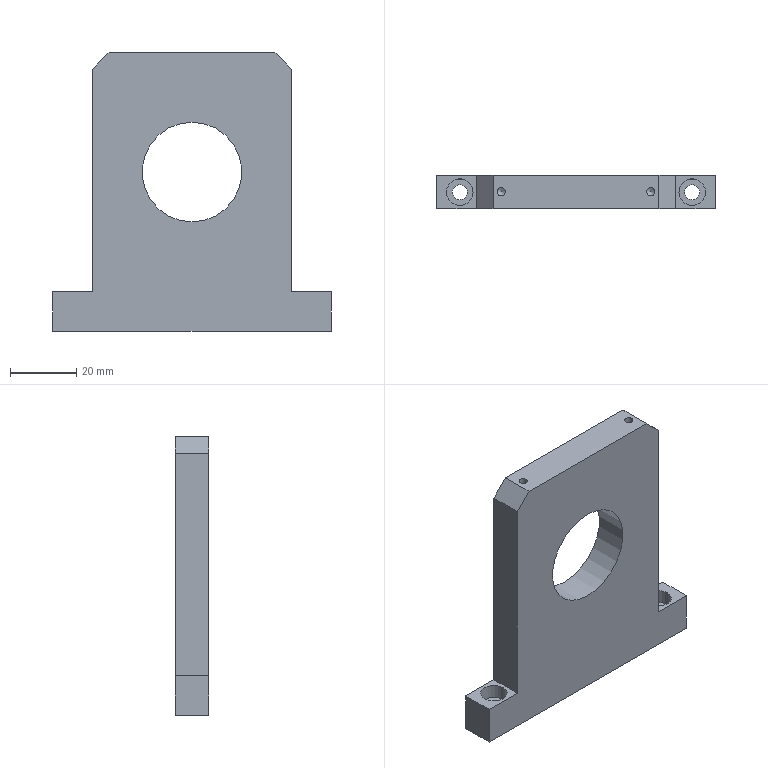Part | NX | 1 solid | 23 faces | box 84 x 10 x 84 mm | volume 45201 mm3 | plane 14 | cylinder 7 | cone 2 | commonest cylinder face diameters 2.5 x2 4.5 x2 8 x2 30 x1
STEP:
#1=CARTESIAN_POINT('',(30.,10.,31.));
#2=VERTEX_POINT('',#1);
#3=CARTESIAN_POINT('',(30.,10.,-36.));
#4=VERTEX_POINT('',#3);
#5=CARTESIAN_POINT('',(30.,10.,36.));
#6=DIRECTION('',(0.,0.,-1.));
#7=VECTOR('',#6,1000.);
#8=LINE('',#5,#7);
#9=EDGE_CURVE('',#2,#4,#8,.T.);
#10=ORIENTED_EDGE('',*,*,#9,.F.);
#11=CARTESIAN_POINT('',(30.,0.,31.));
#12=VERTEX_POINT('',#11);
#13=CARTESIAN_POINT('',(30.,10.,31.));
#14=DIRECTION('',(0.,-1.,0.));
#15=VECTOR('',#14,1000.);
#16=LINE('',#13,#15);
#17=EDGE_CURVE('',#2,#12,#16,.T.);
#18=ORIENTED_EDGE('',*,*,#17,.T.);
#19=CARTESIAN_POINT('',(30.,0.,-36.));
#20=VERTEX_POINT('',#19);
#21=CARTESIAN_POINT('',(30.,0.,36.));
#22=DIRECTION('',(0.,0.,-1.));
#23=VECTOR('',#22,1000.);
#24=LINE('',#21,#23);
#25=EDGE_CURVE('',#12,#20,#24,.T.);
#26=ORIENTED_EDGE('',*,*,#25,.T.);
#27=CARTESIAN_POINT('',(30.,10.,-36.));
#28=DIRECTION('',(0.,-1.,0.));
#29=VECTOR('',#28,1000.);
#30=LINE('',#27,#29);
#31=EDGE_CURVE('',#4,#20,#30,.T.);
#32=ORIENTED_EDGE('',*,*,#31,.F.);
#33=EDGE_LOOP('',(#10,#18,#26,#32));
#34=FACE_BOUND('',#33,.T.);
#35=CARTESIAN_POINT('',(30.,10.,36.));
#36=DIRECTION('',(-1.,0.,0.));
#37=DIRECTION('',(0.,0.,1.));
#38=AXIS2_PLACEMENT_3D('',#35,#36,#37);
#39=PLANE('',#38);
#40=ADVANCED_FACE('',(#34),#39,.F.);
#41=CARTESIAN_POINT('',(-30.,0.,-36.));
#42=VERTEX_POINT('',#41);
#43=CARTESIAN_POINT('',(-30.,0.,31.));
#44=VERTEX_POINT('',#43);
#45=CARTESIAN_POINT('',(-30.,0.,36.));
#46=DIRECTION('',(0.,0.,1.));
#47=VECTOR('',#46,1000.);
#48=LINE('',#45,#47);
#49=EDGE_CURVE('',#42,#44,#48,.T.);
#50=ORIENTED_EDGE('',*,*,#49,.T.);
#51=CARTESIAN_POINT('',(-30.,10.,31.));
#52=VERTEX_POINT('',#51);
#53=CARTESIAN_POINT('',(-30.,10.,31.));
#54=DIRECTION('',(0.,1.,0.));
#55=VECTOR('',#54,1000.);
#56=LINE('',#53,#55);
#57=EDGE_CURVE('',#44,#52,#56,.T.);
#58=ORIENTED_EDGE('',*,*,#57,.T.);
#59=CARTESIAN_POINT('',(-30.,10.,-36.));
#60=VERTEX_POINT('',#59);
#61=CARTESIAN_POINT('',(-30.,10.,36.));
#62=DIRECTION('',(0.,0.,1.));
#63=VECTOR('',#62,1000.);
#64=LINE('',#61,#63);
#65=EDGE_CURVE('',#60,#52,#64,.T.);
#66=ORIENTED_EDGE('',*,*,#65,.F.);
#67=CARTESIAN_POINT('',(-30.,10.,-36.));
#68=DIRECTION('',(0.,-1.,0.));
#69=VECTOR('',#68,1000.);
#70=LINE('',#67,#69);
#71=EDGE_CURVE('',#60,#42,#70,.T.);
#72=ORIENTED_EDGE('',*,*,#71,.T.);
#73=EDGE_LOOP('',(#50,#58,#66,#72));
#74=FACE_BOUND('',#73,.T.);
#75=CARTESIAN_POINT('',(-30.,10.,36.));
#76=DIRECTION('',(1.,0.,0.));
#77=DIRECTION('',(0.,0.,-1.));
#78=AXIS2_PLACEMENT_3D('',#75,#76,#77);
#79=PLANE('',#78);
#80=ADVANCED_FACE('',(#74),#79,.F.);
#81=CARTESIAN_POINT('',(-21.25,5.,36.));
#82=VERTEX_POINT('',#81);
#83=CARTESIAN_POINT('',(-22.5,5.,36.));
#84=DIRECTION('',(0.,0.,1.));
#85=DIRECTION('',(1.,0.,0.));
#86=AXIS2_PLACEMENT_3D('',#83,#84,#85);
#87=CIRCLE('',#86,1.25);
#88=EDGE_CURVE('',#82,#82,#87,.T.);
#89=ORIENTED_EDGE('',*,*,#88,.F.);
#90=EDGE_LOOP('',(#89));
#91=FACE_BOUND('',#90,.T.);
#92=CARTESIAN_POINT('',(23.75,5.,36.));
#93=VERTEX_POINT('',#92);
#94=CARTESIAN_POINT('',(22.5,5.,36.));
#95=DIRECTION('',(0.,0.,1.));
#96=DIRECTION('',(1.,0.,0.));
#97=AXIS2_PLACEMENT_3D('',#94,#95,#96);
#98=CIRCLE('',#97,1.25);
#99=EDGE_CURVE('',#93,#93,#98,.T.);
#100=ORIENTED_EDGE('',*,*,#99,.F.);
#101=EDGE_LOOP('',(#100));
#102=FACE_BOUND('',#101,.T.);
#103=CARTESIAN_POINT('',(-25.,0.,36.));
#104=VERTEX_POINT('',#103);
#105=CARTESIAN_POINT('',(25.,0.,36.));
#106=VERTEX_POINT('',#105);
#107=CARTESIAN_POINT('',(-30.,0.,36.));
#108=DIRECTION('',(1.,0.,0.));
#109=VECTOR('',#108,1000.);
#110=LINE('',#107,#109);
#111=EDGE_CURVE('',#104,#106,#110,.T.);
#112=ORIENTED_EDGE('',*,*,#111,.T.);
#113=CARTESIAN_POINT('',(25.,10.,36.));
#114=VERTEX_POINT('',#113);
#115=CARTESIAN_POINT('',(25.,10.,36.));
#116=DIRECTION('',(0.,1.,0.));
#117=VECTOR('',#116,1000.);
#118=LINE('',#115,#117);
#119=EDGE_CURVE('',#106,#114,#118,.T.);
#120=ORIENTED_EDGE('',*,*,#119,.T.);
#121=CARTESIAN_POINT('',(-25.,10.,36.));
#122=VERTEX_POINT('',#121);
#123=CARTESIAN_POINT('',(-30.,10.,36.));
#124=DIRECTION('',(1.,0.,0.));
#125=VECTOR('',#124,1000.);
#126=LINE('',#123,#125);
#127=EDGE_CURVE('',#122,#114,#126,.T.);
#128=ORIENTED_EDGE('',*,*,#127,.F.);
#129=CARTESIAN_POINT('',(-25.,10.,36.));
#130=DIRECTION('',(0.,-1.,0.));
#131=VECTOR('',#130,1000.);
#132=LINE('',#129,#131);
#133=EDGE_CURVE('',#122,#104,#132,.T.);
#134=ORIENTED_EDGE('',*,*,#133,.T.);
#135=EDGE_LOOP('',(#112,#120,#128,#134));
#136=FACE_BOUND('',#135,.T.);
#137=CARTESIAN_POINT('',(-30.,10.,36.));
#138=DIRECTION('',(0.,0.,-1.));
#139=DIRECTION('',(-1.,0.,0.));
#140=AXIS2_PLACEMENT_3D('',#137,#138,#139);
#141=PLANE('',#140);
#142=ADVANCED_FACE('',(#91,#102,#136),#141,.F.);
#143=CARTESIAN_POINT('',(0.,10.,-15.));
#144=VERTEX_POINT('',#143);
#145=CARTESIAN_POINT('',(0.,10.,0.));
#146=DIRECTION('',(0.,-1.,0.));
#147=DIRECTION('',(0.,0.,-1.));
#148=AXIS2_PLACEMENT_3D('',#145,#146,#147);
#149=CIRCLE('',#148,15.);
#150=EDGE_CURVE('',#144,#144,#149,.T.);
#151=ORIENTED_EDGE('',*,*,#150,.T.);
#152=EDGE_LOOP('',(#151));
#153=FACE_BOUND('',#152,.T.);
#154=ORIENTED_EDGE('',*,*,#127,.T.);
#155=CARTESIAN_POINT('',(30.,10.,31.));
#156=DIRECTION('',(-0.7071,0.,0.7071));
#157=VECTOR('',#156,1000.);
#158=LINE('',#155,#157);
#159=EDGE_CURVE('',#114,#2,#158,.F.);
#160=ORIENTED_EDGE('',*,*,#159,.T.);
#161=ORIENTED_EDGE('',*,*,#9,.T.);
#162=CARTESIAN_POINT('',(42.,10.,-36.));
#163=VERTEX_POINT('',#162);
#164=CARTESIAN_POINT('',(-42.,10.,-36.));
#165=DIRECTION('',(1.,0.,0.));
#166=VECTOR('',#165,1000.);
#167=LINE('',#164,#166);
#168=EDGE_CURVE('',#4,#163,#167,.T.);
#169=ORIENTED_EDGE('',*,*,#168,.T.);
#170=CARTESIAN_POINT('',(42.,10.,-48.));
#171=VERTEX_POINT('',#170);
#172=CARTESIAN_POINT('',(42.,10.,-48.));
#173=DIRECTION('',(0.,0.,-1.));
#174=VECTOR('',#173,1000.);
#175=LINE('',#172,#174);
#176=EDGE_CURVE('',#163,#171,#175,.T.);
#177=ORIENTED_EDGE('',*,*,#176,.T.);
#178=CARTESIAN_POINT('',(-42.,10.,-48.));
#179=VERTEX_POINT('',#178);
#180=CARTESIAN_POINT('',(-42.,10.,-48.));
#181=DIRECTION('',(-1.,0.,0.));
#182=VECTOR('',#181,1000.);
#183=LINE('',#180,#182);
#184=EDGE_CURVE('',#171,#179,#183,.T.);
#185=ORIENTED_EDGE('',*,*,#184,.T.);
#186=CARTESIAN_POINT('',(-42.,10.,-36.));
#187=VERTEX_POINT('',#186);
#188=CARTESIAN_POINT('',(-42.,10.,-48.));
#189=DIRECTION('',(0.,0.,1.));
#190=VECTOR('',#189,1000.);
#191=LINE('',#188,#190);
#192=EDGE_CURVE('',#179,#187,#191,.T.);
#193=ORIENTED_EDGE('',*,*,#192,.T.);
#194=CARTESIAN_POINT('',(-42.,10.,-36.));
#195=DIRECTION('',(1.,0.,0.));
#196=VECTOR('',#195,1000.);
#197=LINE('',#194,#196);
#198=EDGE_CURVE('',#187,#60,#197,.T.);
#199=ORIENTED_EDGE('',*,*,#198,.T.);
#200=ORIENTED_EDGE('',*,*,#65,.T.);
#201=CARTESIAN_POINT('',(-25.,10.,36.));
#202=DIRECTION('',(-0.7071,0.,-0.7071));
#203=VECTOR('',#202,1000.);
#204=LINE('',#201,#203);
#205=EDGE_CURVE('',#52,#122,#204,.F.);
#206=ORIENTED_EDGE('',*,*,#205,.T.);
#207=EDGE_LOOP('',(#154,#160,#161,#169,#177,#185,#193,#199,#200,#206));
#208=FACE_BOUND('',#207,.T.);
#209=CARTESIAN_POINT('',(0.,10.,0.));
#210=DIRECTION('',(0.,-1.,0.));
#211=DIRECTION('',(0.,0.,-1.));
#212=AXIS2_PLACEMENT_3D('',#209,#210,#211);
#213=PLANE('',#212);
#214=ADVANCED_FACE('',(#153,#208),#213,.F.);
#215=CARTESIAN_POINT('',(0.,0.,-15.));
#216=VERTEX_POINT('',#215);
#217=CARTESIAN_POINT('',(0.,0.,0.));
#218=DIRECTION('',(0.,-1.,0.));
#219=DIRECTION('',(0.,0.,-1.));
#220=AXIS2_PLACEMENT_3D('',#217,#218,#219);
#221=CIRCLE('',#220,15.);
#222=EDGE_CURVE('',#216,#216,#221,.T.);
#223=ORIENTED_EDGE('',*,*,#222,.F.);
#224=EDGE_LOOP('',(#223));
#225=FACE_BOUND('',#224,.T.);
#226=ORIENTED_EDGE('',*,*,#25,.F.);
#227=CARTESIAN_POINT('',(30.5,0.,30.5));
#228=DIRECTION('',(0.7071,0.,-0.7071));
#229=VECTOR('',#228,1000.);
#230=LINE('',#227,#229);
#231=EDGE_CURVE('',#12,#106,#230,.F.);
#232=ORIENTED_EDGE('',*,*,#231,.T.);
#233=ORIENTED_EDGE('',*,*,#111,.F.);
#234=CARTESIAN_POINT('',(-30.5,0.,30.5));
#235=DIRECTION('',(0.7071,0.,0.7071));
#236=VECTOR('',#235,1000.);
#237=LINE('',#234,#236);
#238=EDGE_CURVE('',#104,#44,#237,.F.);
#239=ORIENTED_EDGE('',*,*,#238,.T.);
#240=ORIENTED_EDGE('',*,*,#49,.F.);
#241=CARTESIAN_POINT('',(-42.,0.,-36.));
#242=VERTEX_POINT('',#241);
#243=CARTESIAN_POINT('',(-42.,0.,-36.));
#244=DIRECTION('',(1.,0.,0.));
#245=VECTOR('',#244,1000.);
#246=LINE('',#243,#245);
#247=EDGE_CURVE('',#242,#42,#246,.T.);
#248=ORIENTED_EDGE('',*,*,#247,.F.);
#249=CARTESIAN_POINT('',(-42.,0.,-48.));
#250=VERTEX_POINT('',#249);
#251=CARTESIAN_POINT('',(-42.,0.,-48.));
#252=DIRECTION('',(0.,0.,1.));
#253=VECTOR('',#252,1000.);
#254=LINE('',#251,#253);
#255=EDGE_CURVE('',#250,#242,#254,.T.);
#256=ORIENTED_EDGE('',*,*,#255,.F.);
#257=CARTESIAN_POINT('',(42.,0.,-48.));
#258=VERTEX_POINT('',#257);
#259=CARTESIAN_POINT('',(-42.,0.,-48.));
#260=DIRECTION('',(-1.,0.,0.));
#261=VECTOR('',#260,1000.);
#262=LINE('',#259,#261);
#263=EDGE_CURVE('',#258,#250,#262,.T.);
#264=ORIENTED_EDGE('',*,*,#263,.F.);
#265=CARTESIAN_POINT('',(42.,0.,-36.));
#266=VERTEX_POINT('',#265);
#267=CARTESIAN_POINT('',(42.,0.,-48.));
#268=DIRECTION('',(0.,0.,-1.));
#269=VECTOR('',#268,1000.);
#270=LINE('',#267,#269);
#271=EDGE_CURVE('',#266,#258,#270,.T.);
#272=ORIENTED_EDGE('',*,*,#271,.F.);
#273=CARTESIAN_POINT('',(-42.,0.,-36.));
#274=DIRECTION('',(1.,0.,0.));
#275=VECTOR('',#274,1000.);
#276=LINE('',#273,#275);
#277=EDGE_CURVE('',#20,#266,#276,.T.);
#278=ORIENTED_EDGE('',*,*,#277,.F.);
#279=EDGE_LOOP('',(#226,#232,#233,#239,#240,#248,#256,#264,#272,#278));
#280=FACE_BOUND('',#279,.T.);
#281=CARTESIAN_POINT('',(0.,0.,0.));
#282=DIRECTION('',(0.,-1.,0.));
#283=DIRECTION('',(0.,0.,-1.));
#284=AXIS2_PLACEMENT_3D('',#281,#282,#283);
#285=PLANE('',#284);
#286=ADVANCED_FACE('',(#225,#280),#285,.T.);
#287=CARTESIAN_POINT('',(22.5,5.,27.749));
#288=VERTEX_POINT('',#287);
#289=VERTEX_LOOP('',#288);
#290=FACE_BOUND('',#289,.T.);
#291=CARTESIAN_POINT('',(23.75,5.,28.5));
#292=VERTEX_POINT('',#291);
#293=CARTESIAN_POINT('',(22.5,5.,28.5));
#294=DIRECTION('',(0.,0.,1.));
#295=DIRECTION('',(1.,0.,0.));
#296=AXIS2_PLACEMENT_3D('',#293,#294,#295);
#297=CIRCLE('',#296,1.25);
#298=EDGE_CURVE('',#292,#292,#297,.T.);
#299=ORIENTED_EDGE('',*,*,#298,.T.);
#300=EDGE_LOOP('',(#299));
#301=FACE_BOUND('',#300,.T.);
#302=CARTESIAN_POINT('',(22.5,5.,28.5));
#303=DIRECTION('',(0.,0.,1.));
#304=DIRECTION('',(1.,0.,0.));
#305=AXIS2_PLACEMENT_3D('',#302,#303,#304);
#306=CONICAL_SURFACE('',#305,1.25,1.03);
#307=ADVANCED_FACE('',(#290,#301),#306,.F.);
#308=ORIENTED_EDGE('',*,*,#298,.F.);
#309=EDGE_LOOP('',(#308));
#310=FACE_BOUND('',#309,.T.);
#311=ORIENTED_EDGE('',*,*,#99,.T.);
#312=EDGE_LOOP('',(#311));
#313=FACE_BOUND('',#312,.T.);
#314=CARTESIAN_POINT('',(22.5,5.,36.));
#315=DIRECTION('',(0.,0.,1.));
#316=DIRECTION('',(1.,0.,0.));
#317=AXIS2_PLACEMENT_3D('',#314,#315,#316);
#318=CYLINDRICAL_SURFACE('',#317,1.25);
#319=ADVANCED_FACE('',(#310,#313),#318,.F.);
#320=CARTESIAN_POINT('',(-22.5,5.,27.749));
#321=VERTEX_POINT('',#320);
#322=VERTEX_LOOP('',#321);
#323=FACE_BOUND('',#322,.T.);
#324=CARTESIAN_POINT('',(-21.25,5.,28.5));
#325=VERTEX_POINT('',#324);
#326=CARTESIAN_POINT('',(-22.5,5.,28.5));
#327=DIRECTION('',(0.,0.,1.));
#328=DIRECTION('',(1.,0.,0.));
#329=AXIS2_PLACEMENT_3D('',#326,#327,#328);
#330=CIRCLE('',#329,1.25);
#331=EDGE_CURVE('',#325,#325,#330,.T.);
#332=ORIENTED_EDGE('',*,*,#331,.T.);
#333=EDGE_LOOP('',(#332));
#334=FACE_BOUND('',#333,.T.);
#335=CARTESIAN_POINT('',(-22.5,5.,28.5));
#336=DIRECTION('',(0.,0.,1.));
#337=DIRECTION('',(1.,0.,0.));
#338=AXIS2_PLACEMENT_3D('',#335,#336,#337);
#339=CONICAL_SURFACE('',#338,1.25,1.03);
#340=ADVANCED_FACE('',(#323,#334),#339,.F.);
#341=ORIENTED_EDGE('',*,*,#331,.F.);
#342=EDGE_LOOP('',(#341));
#343=FACE_BOUND('',#342,.T.);
#344=ORIENTED_EDGE('',*,*,#88,.T.);
#345=EDGE_LOOP('',(#344));
#346=FACE_BOUND('',#345,.T.);
#347=CARTESIAN_POINT('',(-22.5,5.,36.));
#348=DIRECTION('',(0.,0.,1.));
#349=DIRECTION('',(1.,0.,0.));
#350=AXIS2_PLACEMENT_3D('',#347,#348,#349);
#351=CYLINDRICAL_SURFACE('',#350,1.25);
#352=ADVANCED_FACE('',(#343,#346),#351,.F.);
#353=ORIENTED_EDGE('',*,*,#150,.F.);
#354=EDGE_LOOP('',(#353));
#355=FACE_BOUND('',#354,.T.);
#356=ORIENTED_EDGE('',*,*,#222,.T.);
#357=EDGE_LOOP('',(#356));
#358=FACE_BOUND('',#357,.T.);
#359=CARTESIAN_POINT('',(0.,10.,0.));
#360=DIRECTION('',(0.,-1.,0.));
#361=DIRECTION('',(0.,0.,-1.));
#362=AXIS2_PLACEMENT_3D('',#359,#360,#361);
#363=CYLINDRICAL_SURFACE('',#362,15.);
#364=ADVANCED_FACE('',(#355,#358),#363,.F.);
#365=CARTESIAN_POINT('',(-31.,5.,-36.));
#366=VERTEX_POINT('',#365);
#367=CARTESIAN_POINT('',(-35.,5.,-36.));
#368=DIRECTION('',(0.,0.,1.));
#369=DIRECTION('',(1.,0.,0.));
#370=AXIS2_PLACEMENT_3D('',#367,#368,#369);
#371=CIRCLE('',#370,4.);
#372=EDGE_CURVE('',#366,#366,#371,.T.);
#373=ORIENTED_EDGE('',*,*,#372,.F.);
#374=EDGE_LOOP('',(#373));
#375=FACE_BOUND('',#374,.T.);
#376=ORIENTED_EDGE('',*,*,#71,.F.);
#377=ORIENTED_EDGE('',*,*,#198,.F.);
#378=CARTESIAN_POINT('',(-42.,-84.853,-36.));
#379=DIRECTION('',(0.,1.,0.));
#380=VECTOR('',#379,1000.);
#381=LINE('',#378,#380);
#382=EDGE_CURVE('',#242,#187,#381,.T.);
#383=ORIENTED_EDGE('',*,*,#382,.F.);
#384=ORIENTED_EDGE('',*,*,#247,.T.);
#385=EDGE_LOOP('',(#376,#377,#383,#384));
#386=FACE_BOUND('',#385,.T.);
#387=CARTESIAN_POINT('',(-42.,-84.853,-36.));
#388=DIRECTION('',(0.,0.,1.));
#389=DIRECTION('',(1.,0.,0.));
#390=AXIS2_PLACEMENT_3D('',#387,#388,#389);
#391=PLANE('',#390);
#392=ADVANCED_FACE('',(#375,#386),#391,.T.);
#393=CARTESIAN_POINT('',(-32.75,5.,-48.));
#394=VERTEX_POINT('',#393);
#395=CARTESIAN_POINT('',(-35.,5.,-48.));
#396=DIRECTION('',(0.,0.,1.));
#397=DIRECTION('',(1.,0.,0.));
#398=AXIS2_PLACEMENT_3D('',#395,#396,#397);
#399=CIRCLE('',#398,2.25);
#400=EDGE_CURVE('',#394,#394,#399,.T.);
#401=ORIENTED_EDGE('',*,*,#400,.T.);
#402=EDGE_LOOP('',(#401));
#403=FACE_BOUND('',#402,.T.);
#404=CARTESIAN_POINT('',(37.25,5.,-48.));
#405=VERTEX_POINT('',#404);
#406=CARTESIAN_POINT('',(35.,5.,-48.));
#407=DIRECTION('',(0.,0.,1.));
#408=DIRECTION('',(1.,0.,0.));
#409=AXIS2_PLACEMENT_3D('',#406,#407,#408);
#410=CIRCLE('',#409,2.25);
#411=EDGE_CURVE('',#405,#405,#410,.T.);
#412=ORIENTED_EDGE('',*,*,#411,.T.);
#413=EDGE_LOOP('',(#412));
#414=FACE_BOUND('',#413,.T.);
#415=CARTESIAN_POINT('',(42.,-84.853,-48.));
#416=DIRECTION('',(0.,1.,0.));
#417=VECTOR('',#416,1000.);
#418=LINE('',#415,#417);
#419=EDGE_CURVE('',#258,#171,#418,.T.);
#420=ORIENTED_EDGE('',*,*,#419,.F.);
#421=ORIENTED_EDGE('',*,*,#263,.T.);
#422=CARTESIAN_POINT('',(-42.,-84.853,-48.));
#423=DIRECTION('',(0.,1.,0.));
#424=VECTOR('',#423,1000.);
#425=LINE('',#422,#424);
#426=EDGE_CURVE('',#250,#179,#425,.T.);
#427=ORIENTED_EDGE('',*,*,#426,.T.);
#428=ORIENTED_EDGE('',*,*,#184,.F.);
#429=EDGE_LOOP('',(#420,#421,#427,#428));
#430=FACE_BOUND('',#429,.T.);
#431=CARTESIAN_POINT('',(-42.,-84.853,-48.));
#432=DIRECTION('',(0.,0.,-1.));
#433=DIRECTION('',(-1.,0.,0.));
#434=AXIS2_PLACEMENT_3D('',#431,#432,#433);
#435=PLANE('',#434);
#436=ADVANCED_FACE('',(#403,#414,#430),#435,.T.);
#437=ORIENTED_EDGE('',*,*,#426,.F.);
#438=ORIENTED_EDGE('',*,*,#255,.T.);
#439=ORIENTED_EDGE('',*,*,#382,.T.);
#440=ORIENTED_EDGE('',*,*,#192,.F.);
#441=EDGE_LOOP('',(#437,#438,#439,#440));
#442=FACE_BOUND('',#441,.T.);
#443=CARTESIAN_POINT('',(-42.,-84.853,-48.));
#444=DIRECTION('',(-1.,0.,0.));
#445=DIRECTION('',(0.,0.,1.));
#446=AXIS2_PLACEMENT_3D('',#443,#444,#445);
#447=PLANE('',#446);
#448=ADVANCED_FACE('',(#442),#447,.T.);
#449=CARTESIAN_POINT('',(39.,5.,-36.));
#450=VERTEX_POINT('',#449);
#451=CARTESIAN_POINT('',(35.,5.,-36.));
#452=DIRECTION('',(0.,0.,1.));
#453=DIRECTION('',(1.,0.,0.));
#454=AXIS2_PLACEMENT_3D('',#451,#452,#453);
#455=CIRCLE('',#454,4.);
#456=EDGE_CURVE('',#450,#450,#455,.T.);
#457=ORIENTED_EDGE('',*,*,#456,.F.);
#458=EDGE_LOOP('',(#457));
#459=FACE_BOUND('',#458,.T.);
#460=ORIENTED_EDGE('',*,*,#168,.F.);
#461=ORIENTED_EDGE('',*,*,#31,.T.);
#462=ORIENTED_EDGE('',*,*,#277,.T.);
#463=CARTESIAN_POINT('',(42.,-84.853,-36.));
#464=DIRECTION('',(0.,1.,0.));
#465=VECTOR('',#464,1000.);
#466=LINE('',#463,#465);
#467=EDGE_CURVE('',#266,#163,#466,.T.);
#468=ORIENTED_EDGE('',*,*,#467,.T.);
#469=EDGE_LOOP('',(#460,#461,#462,#468));
#470=FACE_BOUND('',#469,.T.);
#471=CARTESIAN_POINT('',(-42.,-84.853,-36.));
#472=DIRECTION('',(0.,0.,1.));
#473=DIRECTION('',(1.,0.,0.));
#474=AXIS2_PLACEMENT_3D('',#471,#472,#473);
#475=PLANE('',#474);
#476=ADVANCED_FACE('',(#459,#470),#475,.T.);
#477=ORIENTED_EDGE('',*,*,#467,.F.);
#478=ORIENTED_EDGE('',*,*,#271,.T.);
#479=ORIENTED_EDGE('',*,*,#419,.T.);
#480=ORIENTED_EDGE('',*,*,#176,.F.);
#481=EDGE_LOOP('',(#477,#478,#479,#480));
#482=FACE_BOUND('',#481,.T.);
#483=CARTESIAN_POINT('',(42.,-84.853,-48.));
#484=DIRECTION('',(1.,0.,0.));
#485=DIRECTION('',(0.,0.,-1.));
#486=AXIS2_PLACEMENT_3D('',#483,#484,#485);
#487=PLANE('',#486);
#488=ADVANCED_FACE('',(#482),#487,.T.);
#489=ORIENTED_EDGE('',*,*,#411,.F.);
#490=EDGE_LOOP('',(#489));
#491=FACE_BOUND('',#490,.T.);
#492=CARTESIAN_POINT('',(37.25,5.,-40.4));
#493=VERTEX_POINT('',#492);
#494=CARTESIAN_POINT('',(35.,5.,-40.4));
#495=DIRECTION('',(0.,0.,1.));
#496=DIRECTION('',(1.,0.,0.));
#497=AXIS2_PLACEMENT_3D('',#494,#495,#496);
#498=CIRCLE('',#497,2.25);
#499=EDGE_CURVE('',#493,#493,#498,.T.);
#500=ORIENTED_EDGE('',*,*,#499,.T.);
#501=EDGE_LOOP('',(#500));
#502=FACE_BOUND('',#501,.T.);
#503=CARTESIAN_POINT('',(35.,5.,-36.));
#504=DIRECTION('',(0.,0.,1.));
#505=DIRECTION('',(1.,0.,0.));
#506=AXIS2_PLACEMENT_3D('',#503,#504,#505);
#507=CYLINDRICAL_SURFACE('',#506,2.25);
#508=ADVANCED_FACE('',(#491,#502),#507,.F.);
#509=ORIENTED_EDGE('',*,*,#499,.F.);
#510=EDGE_LOOP('',(#509));
#511=FACE_BOUND('',#510,.T.);
#512=CARTESIAN_POINT('',(39.,5.,-40.4));
#513=VERTEX_POINT('',#512);
#514=CARTESIAN_POINT('',(35.,5.,-40.4));
#515=DIRECTION('',(0.,0.,1.));
#516=DIRECTION('',(1.,0.,0.));
#517=AXIS2_PLACEMENT_3D('',#514,#515,#516);
#518=CIRCLE('',#517,4.);
#519=EDGE_CURVE('',#513,#513,#518,.T.);
#520=ORIENTED_EDGE('',*,*,#519,.T.);
#521=EDGE_LOOP('',(#520));
#522=FACE_BOUND('',#521,.T.);
#523=CARTESIAN_POINT('',(37.25,5.,-40.4));
#524=DIRECTION('',(0.,0.,-1.));
#525=DIRECTION('',(-1.,0.,0.));
#526=AXIS2_PLACEMENT_3D('',#523,#524,#525);
#527=PLANE('',#526);
#528=ADVANCED_FACE('',(#511,#522),#527,.F.);
#529=ORIENTED_EDGE('',*,*,#519,.F.);
#530=EDGE_LOOP('',(#529));
#531=FACE_BOUND('',#530,.T.);
#532=ORIENTED_EDGE('',*,*,#456,.T.);
#533=EDGE_LOOP('',(#532));
#534=FACE_BOUND('',#533,.T.);
#535=CARTESIAN_POINT('',(35.,5.,-36.));
#536=DIRECTION('',(0.,0.,1.));
#537=DIRECTION('',(1.,0.,0.));
#538=AXIS2_PLACEMENT_3D('',#535,#536,#537);
#539=CYLINDRICAL_SURFACE('',#538,4.);
#540=ADVANCED_FACE('',(#531,#534),#539,.F.);
#541=ORIENTED_EDGE('',*,*,#400,.F.);
#542=EDGE_LOOP('',(#541));
#543=FACE_BOUND('',#542,.T.);
#544=CARTESIAN_POINT('',(-32.75,5.,-40.4));
#545=VERTEX_POINT('',#544);
#546=CARTESIAN_POINT('',(-35.,5.,-40.4));
#547=DIRECTION('',(0.,0.,1.));
#548=DIRECTION('',(1.,0.,0.));
#549=AXIS2_PLACEMENT_3D('',#546,#547,#548);
#550=CIRCLE('',#549,2.25);
#551=EDGE_CURVE('',#545,#545,#550,.T.);
#552=ORIENTED_EDGE('',*,*,#551,.T.);
#553=EDGE_LOOP('',(#552));
#554=FACE_BOUND('',#553,.T.);
#555=CARTESIAN_POINT('',(-35.,5.,-36.));
#556=DIRECTION('',(0.,0.,1.));
#557=DIRECTION('',(1.,0.,0.));
#558=AXIS2_PLACEMENT_3D('',#555,#556,#557);
#559=CYLINDRICAL_SURFACE('',#558,2.25);
#560=ADVANCED_FACE('',(#543,#554),#559,.F.);
#561=ORIENTED_EDGE('',*,*,#551,.F.);
#562=EDGE_LOOP('',(#561));
#563=FACE_BOUND('',#562,.T.);
#564=CARTESIAN_POINT('',(-31.,5.,-40.4));
#565=VERTEX_POINT('',#564);
#566=CARTESIAN_POINT('',(-35.,5.,-40.4));
#567=DIRECTION('',(0.,0.,1.));
#568=DIRECTION('',(1.,0.,0.));
#569=AXIS2_PLACEMENT_3D('',#566,#567,#568);
#570=CIRCLE('',#569,4.);
#571=EDGE_CURVE('',#565,#565,#570,.T.);
#572=ORIENTED_EDGE('',*,*,#571,.T.);
#573=EDGE_LOOP('',(#572));
#574=FACE_BOUND('',#573,.T.);
#575=CARTESIAN_POINT('',(-32.75,5.,-40.4));
#576=DIRECTION('',(0.,0.,-1.));
#577=DIRECTION('',(-1.,0.,0.));
#578=AXIS2_PLACEMENT_3D('',#575,#576,#577);
#579=PLANE('',#578);
#580=ADVANCED_FACE('',(#563,#574),#579,.F.);
#581=ORIENTED_EDGE('',*,*,#571,.F.);
#582=EDGE_LOOP('',(#581));
#583=FACE_BOUND('',#582,.T.);
#584=ORIENTED_EDGE('',*,*,#372,.T.);
#585=EDGE_LOOP('',(#584));
#586=FACE_BOUND('',#585,.T.);
#587=CARTESIAN_POINT('',(-35.,5.,-36.));
#588=DIRECTION('',(0.,0.,1.));
#589=DIRECTION('',(1.,0.,0.));
#590=AXIS2_PLACEMENT_3D('',#587,#588,#589);
#591=CYLINDRICAL_SURFACE('',#590,4.);
#592=ADVANCED_FACE('',(#583,#586),#591,.F.);
#593=ORIENTED_EDGE('',*,*,#159,.F.);
#594=ORIENTED_EDGE('',*,*,#119,.F.);
#595=ORIENTED_EDGE('',*,*,#231,.F.);
#596=ORIENTED_EDGE('',*,*,#17,.F.);
#597=EDGE_LOOP('',(#593,#594,#595,#596));
#598=FACE_BOUND('',#597,.T.);
#599=CARTESIAN_POINT('',(30.,10.,31.));
#600=DIRECTION('',(-0.7071,0.,-0.7071));
#601=DIRECTION('',(0.,-1.,0.));
#602=AXIS2_PLACEMENT_3D('',#599,#600,#601);
#603=PLANE('',#602);
#604=ADVANCED_FACE('',(#598),#603,.F.);
#605=ORIENTED_EDGE('',*,*,#205,.F.);
#606=ORIENTED_EDGE('',*,*,#57,.F.);
#607=ORIENTED_EDGE('',*,*,#238,.F.);
#608=ORIENTED_EDGE('',*,*,#133,.F.);
#609=EDGE_LOOP('',(#605,#606,#607,#608));
#610=FACE_BOUND('',#609,.T.);
#611=CARTESIAN_POINT('',(-25.,10.,36.));
#612=DIRECTION('',(0.7071,0.,-0.7071));
#613=DIRECTION('',(0.,-1.,0.));
#614=AXIS2_PLACEMENT_3D('',#611,#612,#613);
#615=PLANE('',#614);
#616=ADVANCED_FACE('',(#610),#615,.F.);
#617=CLOSED_SHELL('',(#40,#80,#142,#214,#286,#307,#319,#340,#352,#364,#392,#436,#448,#476,#488,#508,#528,#540,#560,#580,#592,#604,#616));
#618=MANIFOLD_SOLID_BREP('',#617);
#619=(LENGTH_UNIT()NAMED_UNIT(*)SI_UNIT(.MILLI.,.METRE.));
#620=UNCERTAINTY_MEASURE_WITH_UNIT(LENGTH_MEASURE(0.00001),#619,'','');
#621=(NAMED_UNIT(*)PLANE_ANGLE_UNIT()SI_UNIT($,.RADIAN.));
#622=(NAMED_UNIT(*)SI_UNIT($,.STERADIAN.)SOLID_ANGLE_UNIT());
#623=(GEOMETRIC_REPRESENTATION_CONTEXT(3)GLOBAL_UNCERTAINTY_ASSIGNED_CONTEXT((#620))GLOBAL_UNIT_ASSIGNED_CONTEXT((#619,#621,#622))REPRESENTATION_CONTEXT('',''));
#624=ADVANCED_BREP_SHAPE_REPRESENTATION('',(#618),#623);